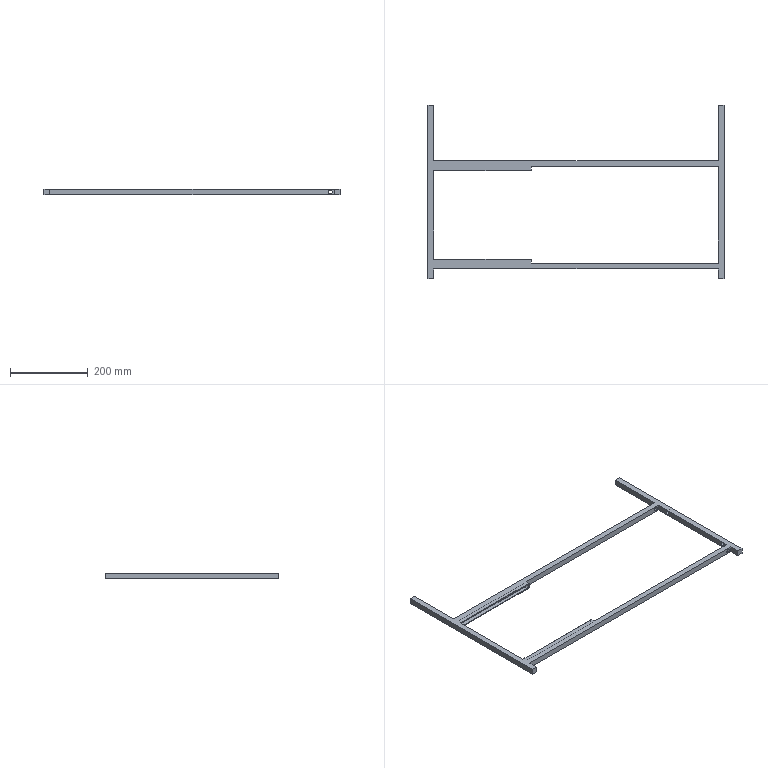Part | SolidWorks | features ICE 4, Cut 1, Extrusion 1 | 1 solid | 40 faces | box 760 x 445 x 15 mm | volume 540712 mm3 | plane 28 | cylinder 12 | commonest cylinder face diameters 10 x8 12 x4
STEP:
#1=CARTESIAN_POINT('',(727.5,-420.,-5.));
#2=VERTEX_POINT('',#1);
#3=CARTESIAN_POINT('',(727.5,-420.,5.));
#4=VERTEX_POINT('',#3);
#5=CARTESIAN_POINT('',(727.5,-420.,0.));
#6=DIRECTION('',(0.,1.,0.));
#7=DIRECTION('',(0.,0.,1.));
#8=AXIS2_PLACEMENT_3D('',#5,#6,#7);
#9=CIRCLE('',#8,5.);
#10=EDGE_CURVE('',#2,#4,#9,.T.);
#11=ORIENTED_EDGE('',*,*,#10,.F.);
#12=CARTESIAN_POINT('',(727.5,-405.,-5.));
#13=VERTEX_POINT('',#12);
#14=CARTESIAN_POINT('',(727.5,-642.5,-5.));
#15=DIRECTION('',(0.,1.,0.));
#16=VECTOR('',#15,1000.);
#17=LINE('',#14,#16);
#18=EDGE_CURVE('',#2,#13,#17,.T.);
#19=ORIENTED_EDGE('',*,*,#18,.T.);
#20=CARTESIAN_POINT('',(727.5,-405.,5.));
#21=VERTEX_POINT('',#20);
#22=CARTESIAN_POINT('',(727.5,-405.,0.));
#23=DIRECTION('',(0.,-1.,0.));
#24=DIRECTION('',(0.,0.,-1.));
#25=AXIS2_PLACEMENT_3D('',#22,#23,#24);
#26=CIRCLE('',#25,5.);
#27=EDGE_CURVE('',#21,#13,#26,.T.);
#28=ORIENTED_EDGE('',*,*,#27,.F.);
#29=CARTESIAN_POINT('',(727.5,-642.5,5.));
#30=DIRECTION('',(0.,1.,0.));
#31=VECTOR('',#30,1000.);
#32=LINE('',#29,#31);
#33=EDGE_CURVE('',#4,#21,#32,.T.);
#34=ORIENTED_EDGE('',*,*,#33,.F.);
#35=EDGE_LOOP('',(#11,#19,#28,#34));
#36=FACE_OUTER_BOUND('',#35,.T.);
#37=CARTESIAN_POINT('',(727.5,-642.5,0.));
#38=DIRECTION('',(0.,1.,0.));
#39=DIRECTION('',(0.,0.,1.));
#40=AXIS2_PLACEMENT_3D('',#37,#38,#39);
#41=CYLINDRICAL_SURFACE('',#40,5.);
#42=ADVANCED_FACE('',(#36),#41,.F.);
#43=CARTESIAN_POINT('',(727.5,-157.5,-5.));
#44=VERTEX_POINT('',#43);
#45=CARTESIAN_POINT('',(727.5,-157.5,5.));
#46=VERTEX_POINT('',#45);
#47=CARTESIAN_POINT('',(727.5,-157.5,0.));
#48=DIRECTION('',(0.,1.,0.));
#49=DIRECTION('',(0.,0.,1.));
#50=AXIS2_PLACEMENT_3D('',#47,#48,#49);
#51=CIRCLE('',#50,5.);
#52=EDGE_CURVE('',#44,#46,#51,.T.);
#53=ORIENTED_EDGE('',*,*,#52,.F.);
#54=CARTESIAN_POINT('',(727.5,-142.5,-5.));
#55=VERTEX_POINT('',#54);
#56=CARTESIAN_POINT('',(727.5,-642.5,-5.));
#57=DIRECTION('',(0.,1.,0.));
#58=VECTOR('',#57,1000.);
#59=LINE('',#56,#58);
#60=EDGE_CURVE('',#44,#55,#59,.T.);
#61=ORIENTED_EDGE('',*,*,#60,.T.);
#62=CARTESIAN_POINT('',(727.5,-142.5,5.));
#63=VERTEX_POINT('',#62);
#64=CARTESIAN_POINT('',(727.5,-142.5,0.));
#65=DIRECTION('',(0.,1.,0.));
#66=DIRECTION('',(0.,0.,1.));
#67=AXIS2_PLACEMENT_3D('',#64,#65,#66);
#68=CIRCLE('',#67,5.);
#69=EDGE_CURVE('',#55,#63,#68,.T.);
#70=ORIENTED_EDGE('',*,*,#69,.T.);
#71=CARTESIAN_POINT('',(727.5,-642.5,5.));
#72=DIRECTION('',(0.,1.,0.));
#73=VECTOR('',#72,1000.);
#74=LINE('',#71,#73);
#75=EDGE_CURVE('',#46,#63,#74,.T.);
#76=ORIENTED_EDGE('',*,*,#75,.F.);
#77=EDGE_LOOP('',(#53,#61,#70,#76));
#78=FACE_OUTER_BOUND('',#77,.T.);
#79=CARTESIAN_POINT('',(727.5,-642.5,0.));
#80=DIRECTION('',(0.,1.,0.));
#81=DIRECTION('',(0.,0.,1.));
#82=AXIS2_PLACEMENT_3D('',#79,#80,#81);
#83=CYLINDRICAL_SURFACE('',#82,5.);
#84=ADVANCED_FACE('',(#78),#83,.F.);
#85=CARTESIAN_POINT('',(752.5,-190.,-5.));
#86=VERTEX_POINT('',#85);
#87=CARTESIAN_POINT('',(752.5,-190.,5.));
#88=VERTEX_POINT('',#87);
#89=CARTESIAN_POINT('',(752.5,-190.,0.));
#90=DIRECTION('',(-1.,0.,0.));
#91=DIRECTION('',(0.,0.,-1.));
#92=AXIS2_PLACEMENT_3D('',#89,#90,#91);
#93=CIRCLE('',#92,5.);
#94=EDGE_CURVE('',#86,#88,#93,.T.);
#95=ORIENTED_EDGE('',*,*,#94,.F.);
#96=CARTESIAN_POINT('',(737.5,-190.,-5.));
#97=VERTEX_POINT('',#96);
#98=CARTESIAN_POINT('',(907.5,-190.,-5.));
#99=DIRECTION('',(-1.,0.,0.));
#100=VECTOR('',#99,1000.);
#101=LINE('',#98,#100);
#102=EDGE_CURVE('',#86,#97,#101,.T.);
#103=ORIENTED_EDGE('',*,*,#102,.T.);
#104=CARTESIAN_POINT('',(737.5,-190.,5.));
#105=VERTEX_POINT('',#104);
#106=CARTESIAN_POINT('',(737.5,-190.,0.));
#107=DIRECTION('',(1.,0.,0.));
#108=DIRECTION('',(0.,0.,1.));
#109=AXIS2_PLACEMENT_3D('',#106,#107,#108);
#110=CIRCLE('',#109,5.);
#111=EDGE_CURVE('',#105,#97,#110,.T.);
#112=ORIENTED_EDGE('',*,*,#111,.F.);
#113=CARTESIAN_POINT('',(907.5,-190.,5.));
#114=DIRECTION('',(-1.,0.,0.));
#115=VECTOR('',#114,1000.);
#116=LINE('',#113,#115);
#117=EDGE_CURVE('',#88,#105,#116,.T.);
#118=ORIENTED_EDGE('',*,*,#117,.F.);
#119=EDGE_LOOP('',(#95,#103,#112,#118));
#120=FACE_OUTER_BOUND('',#119,.T.);
#121=CARTESIAN_POINT('',(907.5,-190.,0.));
#122=DIRECTION('',(-1.,0.,0.));
#123=DIRECTION('',(0.,0.,1.));
#124=AXIS2_PLACEMENT_3D('',#121,#122,#123);
#125=CYLINDRICAL_SURFACE('',#124,5.);
#126=ADVANCED_FACE('',(#120),#125,.F.);
#127=CARTESIAN_POINT('',(752.5,-390.,-5.));
#128=VERTEX_POINT('',#127);
#129=CARTESIAN_POINT('',(752.5,-390.,5.));
#130=VERTEX_POINT('',#129);
#131=CARTESIAN_POINT('',(752.5,-390.,0.));
#132=DIRECTION('',(-1.,0.,0.));
#133=DIRECTION('',(0.,0.,-1.));
#134=AXIS2_PLACEMENT_3D('',#131,#132,#133);
#135=CIRCLE('',#134,5.);
#136=EDGE_CURVE('',#128,#130,#135,.T.);
#137=ORIENTED_EDGE('',*,*,#136,.F.);
#138=CARTESIAN_POINT('',(737.5,-390.,-5.));
#139=VERTEX_POINT('',#138);
#140=CARTESIAN_POINT('',(907.5,-390.,-5.));
#141=DIRECTION('',(-1.,0.,0.));
#142=VECTOR('',#141,1000.);
#143=LINE('',#140,#142);
#144=EDGE_CURVE('',#128,#139,#143,.T.);
#145=ORIENTED_EDGE('',*,*,#144,.T.);
#146=CARTESIAN_POINT('',(737.5,-390.,5.));
#147=VERTEX_POINT('',#146);
#148=CARTESIAN_POINT('',(737.5,-390.,0.));
#149=DIRECTION('',(1.,0.,0.));
#150=DIRECTION('',(0.,0.,1.));
#151=AXIS2_PLACEMENT_3D('',#148,#149,#150);
#152=CIRCLE('',#151,5.);
#153=EDGE_CURVE('',#147,#139,#152,.T.);
#154=ORIENTED_EDGE('',*,*,#153,.F.);
#155=CARTESIAN_POINT('',(907.5,-390.,5.));
#156=DIRECTION('',(-1.,0.,0.));
#157=VECTOR('',#156,1000.);
#158=LINE('',#155,#157);
#159=EDGE_CURVE('',#130,#147,#158,.T.);
#160=ORIENTED_EDGE('',*,*,#159,.F.);
#161=EDGE_LOOP('',(#137,#145,#154,#160));
#162=FACE_OUTER_BOUND('',#161,.T.);
#163=CARTESIAN_POINT('',(907.5,-390.,0.));
#164=DIRECTION('',(-1.,0.,0.));
#165=DIRECTION('',(0.,0.,1.));
#166=AXIS2_PLACEMENT_3D('',#163,#164,#165);
#167=CYLINDRICAL_SURFACE('',#166,5.);
#168=ADVANCED_FACE('',(#162),#167,.F.);
#169=CARTESIAN_POINT('',(727.5,-157.5,0.));
#170=DIRECTION('',(0.,1.,0.));
#171=DIRECTION('',(0.,0.,1.));
#172=AXIS2_PLACEMENT_3D('',#169,#170,#171);
#173=CIRCLE('',#172,5.);
#174=EDGE_CURVE('',#46,#44,#173,.T.);
#175=ORIENTED_EDGE('',*,*,#174,.T.);
#176=ORIENTED_EDGE('',*,*,#52,.T.);
#177=EDGE_LOOP('',(#175,#176));
#178=FACE_BOUND('',#177,.T.);
#179=CARTESIAN_POINT('',(257.5,-157.5,-7.5));
#180=VERTEX_POINT('',#179);
#181=CARTESIAN_POINT('',(257.5,-157.5,7.5));
#182=VERTEX_POINT('',#181);
#183=CARTESIAN_POINT('',(257.5,-157.5,0.));
#184=DIRECTION('',(0.,0.,1.));
#185=VECTOR('',#184,1000.);
#186=LINE('',#183,#185);
#187=EDGE_CURVE('',#180,#182,#186,.T.);
#188=ORIENTED_EDGE('',*,*,#187,.F.);
#189=CARTESIAN_POINT('',(737.5,-157.5,-7.5));
#190=VERTEX_POINT('',#189);
#191=CARTESIAN_POINT('',(758.713,-157.5,-7.5));
#192=DIRECTION('',(-1.,0.,0.));
#193=VECTOR('',#192,1000.);
#194=LINE('',#191,#193);
#195=EDGE_CURVE('',#190,#180,#194,.T.);
#196=ORIENTED_EDGE('',*,*,#195,.F.);
#197=CARTESIAN_POINT('',(737.5,-157.5,7.5));
#198=VERTEX_POINT('',#197);
#199=CARTESIAN_POINT('',(737.5,-157.5,7.5));
#200=DIRECTION('',(0.,0.,1.));
#201=VECTOR('',#200,1000.);
#202=LINE('',#199,#201);
#203=EDGE_CURVE('',#190,#198,#202,.T.);
#204=ORIENTED_EDGE('',*,*,#203,.T.);
#205=CARTESIAN_POINT('',(758.713,-157.5,7.5));
#206=DIRECTION('',(-1.,0.,0.));
#207=VECTOR('',#206,1000.);
#208=LINE('',#205,#207);
#209=EDGE_CURVE('',#198,#182,#208,.T.);
#210=ORIENTED_EDGE('',*,*,#209,.T.);
#211=EDGE_LOOP('',(#188,#196,#204,#210));
#212=FACE_OUTER_BOUND('',#211,.T.);
#213=CARTESIAN_POINT('',(758.713,-157.5,7.5));
#214=DIRECTION('',(0.,1.,0.));
#215=DIRECTION('',(0.,0.,1.));
#216=AXIS2_PLACEMENT_3D('',#213,#214,#215);
#217=PLANE('',#216);
#218=ADVANCED_FACE('',(#178,#212),#217,.F.);
#219=ORIENTED_EDGE('',*,*,#27,.T.);
#220=CARTESIAN_POINT('',(727.5,-405.,0.));
#221=DIRECTION('',(0.,-1.,0.));
#222=DIRECTION('',(0.,0.,-1.));
#223=AXIS2_PLACEMENT_3D('',#220,#221,#222);
#224=CIRCLE('',#223,5.);
#225=EDGE_CURVE('',#13,#21,#224,.T.);
#226=ORIENTED_EDGE('',*,*,#225,.T.);
#227=EDGE_LOOP('',(#219,#226));
#228=FACE_BOUND('',#227,.T.);
#229=CARTESIAN_POINT('',(737.5,-405.,-7.5));
#230=VERTEX_POINT('',#229);
#231=CARTESIAN_POINT('',(257.5,-405.,-7.5));
#232=VERTEX_POINT('',#231);
#233=CARTESIAN_POINT('',(758.713,-405.,-7.5));
#234=DIRECTION('',(-1.,0.,0.));
#235=VECTOR('',#234,1000.);
#236=LINE('',#233,#235);
#237=EDGE_CURVE('',#230,#232,#236,.T.);
#238=ORIENTED_EDGE('',*,*,#237,.T.);
#239=CARTESIAN_POINT('',(257.5,-405.,7.5));
#240=VERTEX_POINT('',#239);
#241=CARTESIAN_POINT('',(257.5,-405.,0.));
#242=DIRECTION('',(0.,0.,1.));
#243=VECTOR('',#242,1000.);
#244=LINE('',#241,#243);
#245=EDGE_CURVE('',#232,#240,#244,.T.);
#246=ORIENTED_EDGE('',*,*,#245,.T.);
#247=CARTESIAN_POINT('',(737.5,-405.,7.5));
#248=VERTEX_POINT('',#247);
#249=CARTESIAN_POINT('',(758.713,-405.,7.5));
#250=DIRECTION('',(-1.,0.,0.));
#251=VECTOR('',#250,1000.);
#252=LINE('',#249,#251);
#253=EDGE_CURVE('',#248,#240,#252,.T.);
#254=ORIENTED_EDGE('',*,*,#253,.F.);
#255=CARTESIAN_POINT('',(737.5,-405.,7.5));
#256=DIRECTION('',(0.,0.,-1.));
#257=VECTOR('',#256,1000.);
#258=LINE('',#255,#257);
#259=EDGE_CURVE('',#248,#230,#258,.T.);
#260=ORIENTED_EDGE('',*,*,#259,.T.);
#261=EDGE_LOOP('',(#238,#246,#254,#260));
#262=FACE_OUTER_BOUND('',#261,.T.);
#263=CARTESIAN_POINT('',(758.713,-405.,7.5));
#264=DIRECTION('',(0.,-1.,0.));
#265=DIRECTION('',(0.,0.,-1.));
#266=AXIS2_PLACEMENT_3D('',#263,#264,#265);
#267=PLANE('',#266);
#268=ADVANCED_FACE('',(#228,#262),#267,.F.);
#269=CARTESIAN_POINT('',(7.5,-167.5,7.5));
#270=VERTEX_POINT('',#269);
#271=CARTESIAN_POINT('',(7.5,-167.5,-7.5));
#272=VERTEX_POINT('',#271);
#273=CARTESIAN_POINT('',(7.5,-167.5,0.));
#274=DIRECTION('',(0.,0.,-1.));
#275=VECTOR('',#274,1000.);
#276=LINE('',#273,#275);
#277=EDGE_CURVE('',#270,#272,#276,.T.);
#278=ORIENTED_EDGE('',*,*,#277,.F.);
#279=CARTESIAN_POINT('',(7.5,-395.,7.5));
#280=VERTEX_POINT('',#279);
#281=CARTESIAN_POINT('',(7.5,-445.,7.5));
#282=DIRECTION('',(0.,1.,0.));
#283=VECTOR('',#282,1000.);
#284=LINE('',#281,#283);
#285=EDGE_CURVE('',#280,#270,#284,.T.);
#286=ORIENTED_EDGE('',*,*,#285,.F.);
#287=CARTESIAN_POINT('',(7.5,-395.,-7.5));
#288=VERTEX_POINT('',#287);
#289=CARTESIAN_POINT('',(7.5,-395.,0.));
#290=DIRECTION('',(0.,0.,1.));
#291=VECTOR('',#290,1000.);
#292=LINE('',#289,#291);
#293=EDGE_CURVE('',#288,#280,#292,.T.);
#294=ORIENTED_EDGE('',*,*,#293,.F.);
#295=CARTESIAN_POINT('',(7.5,-445.,-7.5));
#296=DIRECTION('',(0.,1.,0.));
#297=VECTOR('',#296,1000.);
#298=LINE('',#295,#297);
#299=EDGE_CURVE('',#288,#272,#298,.T.);
#300=ORIENTED_EDGE('',*,*,#299,.T.);
#301=EDGE_LOOP('',(#278,#286,#294,#300));
#302=FACE_OUTER_BOUND('',#301,.T.);
#303=CARTESIAN_POINT('',(7.5,-445.,-7.5));
#304=DIRECTION('',(1.,0.,0.));
#305=DIRECTION('',(0.,0.,-1.));
#306=AXIS2_PLACEMENT_3D('',#303,#304,#305);
#307=PLANE('',#306);
#308=ADVANCED_FACE('',(#302),#307,.T.);
#309=CARTESIAN_POINT('',(7.5,-142.5,7.5));
#310=VERTEX_POINT('',#309);
#311=CARTESIAN_POINT('',(7.5,0.,7.5));
#312=VERTEX_POINT('',#311);
#313=CARTESIAN_POINT('',(7.5,-445.,7.5));
#314=DIRECTION('',(0.,1.,0.));
#315=VECTOR('',#314,1000.);
#316=LINE('',#313,#315);
#317=EDGE_CURVE('',#310,#312,#316,.T.);
#318=ORIENTED_EDGE('',*,*,#317,.F.);
#319=CARTESIAN_POINT('',(7.5,-142.5,-7.5));
#320=VERTEX_POINT('',#319);
#321=CARTESIAN_POINT('',(7.5,-142.5,7.5));
#322=DIRECTION('',(0.,0.,1.));
#323=VECTOR('',#322,1000.);
#324=LINE('',#321,#323);
#325=EDGE_CURVE('',#320,#310,#324,.T.);
#326=ORIENTED_EDGE('',*,*,#325,.F.);
#327=CARTESIAN_POINT('',(7.5,0.,-7.5));
#328=VERTEX_POINT('',#327);
#329=CARTESIAN_POINT('',(7.5,-445.,-7.5));
#330=DIRECTION('',(0.,1.,0.));
#331=VECTOR('',#330,1000.);
#332=LINE('',#329,#331);
#333=EDGE_CURVE('',#320,#328,#332,.T.);
#334=ORIENTED_EDGE('',*,*,#333,.T.);
#335=CARTESIAN_POINT('',(7.5,0.,-7.5));
#336=DIRECTION('',(0.,0.,-1.));
#337=VECTOR('',#336,1000.);
#338=LINE('',#335,#337);
#339=EDGE_CURVE('',#312,#328,#338,.T.);
#340=ORIENTED_EDGE('',*,*,#339,.F.);
#341=EDGE_LOOP('',(#318,#326,#334,#340));
#342=FACE_OUTER_BOUND('',#341,.T.);
#343=CARTESIAN_POINT('',(7.5,-445.,-7.5));
#344=DIRECTION('',(1.,0.,0.));
#345=DIRECTION('',(0.,0.,-1.));
#346=AXIS2_PLACEMENT_3D('',#343,#344,#345);
#347=PLANE('',#346);
#348=ADVANCED_FACE('',(#342),#347,.T.);
#349=ORIENTED_EDGE('',*,*,#111,.T.);
#350=CARTESIAN_POINT('',(737.5,-190.,0.));
#351=DIRECTION('',(1.,0.,0.));
#352=DIRECTION('',(0.,0.,1.));
#353=AXIS2_PLACEMENT_3D('',#350,#351,#352);
#354=CIRCLE('',#353,5.);
#355=EDGE_CURVE('',#97,#105,#354,.T.);
#356=ORIENTED_EDGE('',*,*,#355,.T.);
#357=EDGE_LOOP('',(#349,#356));
#358=FACE_BOUND('',#357,.T.);
#359=ORIENTED_EDGE('',*,*,#153,.T.);
#360=CARTESIAN_POINT('',(737.5,-390.,0.));
#361=DIRECTION('',(1.,0.,0.));
#362=DIRECTION('',(0.,0.,1.));
#363=AXIS2_PLACEMENT_3D('',#360,#361,#362);
#364=CIRCLE('',#363,5.);
#365=EDGE_CURVE('',#139,#147,#364,.T.);
#366=ORIENTED_EDGE('',*,*,#365,.T.);
#367=EDGE_LOOP('',(#359,#366));
#368=FACE_BOUND('',#367,.T.);
#369=CARTESIAN_POINT('',(737.5,-445.,7.5));
#370=DIRECTION('',(0.,1.,0.));
#371=VECTOR('',#370,1000.);
#372=LINE('',#369,#371);
#373=EDGE_CURVE('',#248,#198,#372,.T.);
#374=ORIENTED_EDGE('',*,*,#373,.T.);
#375=ORIENTED_EDGE('',*,*,#203,.F.);
#376=CARTESIAN_POINT('',(737.5,-445.,-7.5));
#377=DIRECTION('',(0.,1.,0.));
#378=VECTOR('',#377,1000.);
#379=LINE('',#376,#378);
#380=EDGE_CURVE('',#230,#190,#379,.T.);
#381=ORIENTED_EDGE('',*,*,#380,.F.);
#382=ORIENTED_EDGE('',*,*,#259,.F.);
#383=EDGE_LOOP('',(#374,#375,#381,#382));
#384=FACE_OUTER_BOUND('',#383,.T.);
#385=CARTESIAN_POINT('',(737.5,-445.,-7.5));
#386=DIRECTION('',(-1.,0.,0.));
#387=DIRECTION('',(0.,0.,1.));
#388=AXIS2_PLACEMENT_3D('',#385,#386,#387);
#389=PLANE('',#388);
#390=ADVANCED_FACE('',(#358,#368,#384),#389,.T.);
#391=CARTESIAN_POINT('',(737.5,-142.5,-7.5));
#392=VERTEX_POINT('',#391);
#393=CARTESIAN_POINT('',(737.5,0.,-7.5));
#394=VERTEX_POINT('',#393);
#395=CARTESIAN_POINT('',(737.5,-445.,-7.5));
#396=DIRECTION('',(0.,1.,0.));
#397=VECTOR('',#396,1000.);
#398=LINE('',#395,#397);
#399=EDGE_CURVE('',#392,#394,#398,.T.);
#400=ORIENTED_EDGE('',*,*,#399,.F.);
#401=CARTESIAN_POINT('',(737.5,-142.5,7.5));
#402=VERTEX_POINT('',#401);
#403=CARTESIAN_POINT('',(737.5,-142.5,7.5));
#404=DIRECTION('',(0.,0.,-1.));
#405=VECTOR('',#404,1000.);
#406=LINE('',#403,#405);
#407=EDGE_CURVE('',#402,#392,#406,.T.);
#408=ORIENTED_EDGE('',*,*,#407,.F.);
#409=CARTESIAN_POINT('',(737.5,0.,7.5));
#410=VERTEX_POINT('',#409);
#411=CARTESIAN_POINT('',(737.5,-445.,7.5));
#412=DIRECTION('',(0.,1.,0.));
#413=VECTOR('',#412,1000.);
#414=LINE('',#411,#413);
#415=EDGE_CURVE('',#402,#410,#414,.T.);
#416=ORIENTED_EDGE('',*,*,#415,.T.);
#417=CARTESIAN_POINT('',(737.5,0.,-7.5));
#418=DIRECTION('',(0.,0.,1.));
#419=VECTOR('',#418,1000.);
#420=LINE('',#417,#419);
#421=EDGE_CURVE('',#394,#410,#420,.T.);
#422=ORIENTED_EDGE('',*,*,#421,.F.);
#423=EDGE_LOOP('',(#400,#408,#416,#422));
#424=FACE_OUTER_BOUND('',#423,.T.);
#425=CARTESIAN_POINT('',(737.5,-445.,-7.5));
#426=DIRECTION('',(-1.,0.,0.));
#427=DIRECTION('',(0.,0.,1.));
#428=AXIS2_PLACEMENT_3D('',#425,#426,#427);
#429=PLANE('',#428);
#430=ADVANCED_FACE('',(#424),#429,.T.);
#431=CARTESIAN_POINT('',(7.5,-420.,7.5));
#432=VERTEX_POINT('',#431);
#433=CARTESIAN_POINT('',(7.5,-420.,-7.5));
#434=VERTEX_POINT('',#433);
#435=CARTESIAN_POINT('',(7.5,-420.,7.5));
#436=DIRECTION('',(0.,0.,-1.));
#437=VECTOR('',#436,1000.);
#438=LINE('',#435,#437);
#439=EDGE_CURVE('',#432,#434,#438,.T.);
#440=ORIENTED_EDGE('',*,*,#439,.F.);
#441=CARTESIAN_POINT('',(7.5,-445.,7.5));
#442=VERTEX_POINT('',#441);
#443=CARTESIAN_POINT('',(7.5,-445.,7.5));
#444=DIRECTION('',(0.,1.,0.));
#445=VECTOR('',#444,1000.);
#446=LINE('',#443,#445);
#447=EDGE_CURVE('',#442,#432,#446,.T.);
#448=ORIENTED_EDGE('',*,*,#447,.F.);
#449=CARTESIAN_POINT('',(7.5,-445.,-7.5));
#450=VERTEX_POINT('',#449);
#451=CARTESIAN_POINT('',(7.5,-445.,-7.5));
#452=DIRECTION('',(0.,0.,-1.));
#453=VECTOR('',#452,1000.);
#454=LINE('',#451,#453);
#455=EDGE_CURVE('',#442,#450,#454,.T.);
#456=ORIENTED_EDGE('',*,*,#455,.T.);
#457=CARTESIAN_POINT('',(7.5,-445.,-7.5));
#458=DIRECTION('',(0.,1.,0.));
#459=VECTOR('',#458,1000.);
#460=LINE('',#457,#459);
#461=EDGE_CURVE('',#450,#434,#460,.T.);
#462=ORIENTED_EDGE('',*,*,#461,.T.);
#463=EDGE_LOOP('',(#440,#448,#456,#462));
#464=FACE_OUTER_BOUND('',#463,.T.);
#465=CARTESIAN_POINT('',(7.5,-445.,-7.5));
#466=DIRECTION('',(1.,0.,0.));
#467=DIRECTION('',(0.,0.,-1.));
#468=AXIS2_PLACEMENT_3D('',#465,#466,#467);
#469=PLANE('',#468);
#470=ADVANCED_FACE('',(#464),#469,.T.);
#471=CARTESIAN_POINT('',(257.5,-395.,7.5));
#472=VERTEX_POINT('',#471);
#473=CARTESIAN_POINT('',(0.,-395.,7.5));
#474=DIRECTION('',(1.,0.,0.));
#475=VECTOR('',#474,1000.);
#476=LINE('',#473,#475);
#477=EDGE_CURVE('',#280,#472,#476,.T.);
#478=ORIENTED_EDGE('',*,*,#477,.F.);
#479=ORIENTED_EDGE('',*,*,#285,.T.);
#480=CARTESIAN_POINT('',(257.5,-167.5,7.5));
#481=VERTEX_POINT('',#480);
#482=CARTESIAN_POINT('',(0.,-167.5,7.5));
#483=DIRECTION('',(-1.,0.,0.));
#484=VECTOR('',#483,1000.);
#485=LINE('',#482,#484);
#486=EDGE_CURVE('',#481,#270,#485,.T.);
#487=ORIENTED_EDGE('',*,*,#486,.F.);
#488=CARTESIAN_POINT('',(257.5,-167.5,7.5));
#489=DIRECTION('',(0.,1.,0.));
#490=VECTOR('',#489,1000.);
#491=LINE('',#488,#490);
#492=EDGE_CURVE('',#481,#182,#491,.T.);
#493=ORIENTED_EDGE('',*,*,#492,.T.);
#494=ORIENTED_EDGE('',*,*,#209,.F.);
#495=ORIENTED_EDGE('',*,*,#373,.F.);
#496=ORIENTED_EDGE('',*,*,#253,.T.);
#497=CARTESIAN_POINT('',(257.5,-395.,7.5));
#498=DIRECTION('',(0.,-1.,0.));
#499=VECTOR('',#498,1000.);
#500=LINE('',#497,#499);
#501=EDGE_CURVE('',#472,#240,#500,.T.);
#502=ORIENTED_EDGE('',*,*,#501,.F.);
#503=EDGE_LOOP('',(#478,#479,#487,#493,#494,#495,#496,#502));
#504=FACE_BOUND('',#503,.T.);
#505=CARTESIAN_POINT('',(-7.5,0.,7.5));
#506=VERTEX_POINT('',#505);
#507=CARTESIAN_POINT('',(-7.5,0.,7.5));
#508=DIRECTION('',(1.,0.,0.));
#509=VECTOR('',#508,1000.);
#510=LINE('',#507,#509);
#511=EDGE_CURVE('',#506,#312,#510,.T.);
#512=ORIENTED_EDGE('',*,*,#511,.F.);
#513=CARTESIAN_POINT('',(-7.5,-445.,7.5));
#514=VERTEX_POINT('',#513);
#515=CARTESIAN_POINT('',(-7.5,-445.,7.5));
#516=DIRECTION('',(0.,1.,0.));
#517=VECTOR('',#516,1000.);
#518=LINE('',#515,#517);
#519=EDGE_CURVE('',#514,#506,#518,.T.);
#520=ORIENTED_EDGE('',*,*,#519,.F.);
#521=CARTESIAN_POINT('',(-7.5,-445.,7.5));
#522=DIRECTION('',(1.,0.,0.));
#523=VECTOR('',#522,1000.);
#524=LINE('',#521,#523);
#525=EDGE_CURVE('',#514,#442,#524,.T.);
#526=ORIENTED_EDGE('',*,*,#525,.T.);
#527=ORIENTED_EDGE('',*,*,#447,.T.);
#528=CARTESIAN_POINT('',(737.5,-420.,7.5));
#529=VERTEX_POINT('',#528);
#530=CARTESIAN_POINT('',(758.713,-420.,7.5));
#531=DIRECTION('',(-1.,0.,0.));
#532=VECTOR('',#531,1000.);
#533=LINE('',#530,#532);
#534=EDGE_CURVE('',#529,#432,#533,.T.);
#535=ORIENTED_EDGE('',*,*,#534,.F.);
#536=CARTESIAN_POINT('',(737.5,-445.,7.5));
#537=VERTEX_POINT('',#536);
#538=CARTESIAN_POINT('',(737.5,-445.,7.5));
#539=DIRECTION('',(0.,1.,0.));
#540=VECTOR('',#539,1000.);
#541=LINE('',#538,#540);
#542=EDGE_CURVE('',#537,#529,#541,.T.);
#543=ORIENTED_EDGE('',*,*,#542,.F.);
#544=CARTESIAN_POINT('',(752.5,-445.,7.5));
#545=VERTEX_POINT('',#544);
#546=CARTESIAN_POINT('',(752.5,-445.,7.5));
#547=DIRECTION('',(1.,0.,0.));
#548=VECTOR('',#547,1000.);
#549=LINE('',#546,#548);
#550=EDGE_CURVE('',#537,#545,#549,.T.);
#551=ORIENTED_EDGE('',*,*,#550,.T.);
#552=CARTESIAN_POINT('',(752.5,0.,7.5));
#553=VERTEX_POINT('',#552);
#554=CARTESIAN_POINT('',(752.5,-445.,7.5));
#555=DIRECTION('',(0.,1.,0.));
#556=VECTOR('',#555,1000.);
#557=LINE('',#554,#556);
#558=EDGE_CURVE('',#545,#553,#557,.T.);
#559=ORIENTED_EDGE('',*,*,#558,.T.);
#560=CARTESIAN_POINT('',(752.5,0.,7.5));
#561=DIRECTION('',(1.,0.,0.));
#562=VECTOR('',#561,1000.);
#563=LINE('',#560,#562);
#564=EDGE_CURVE('',#410,#553,#563,.T.);
#565=ORIENTED_EDGE('',*,*,#564,.F.);
#566=ORIENTED_EDGE('',*,*,#415,.F.);
#567=CARTESIAN_POINT('',(758.713,-142.5,7.5));
#568=DIRECTION('',(-1.,0.,0.));
#569=VECTOR('',#568,1000.);
#570=LINE('',#567,#569);
#571=EDGE_CURVE('',#402,#310,#570,.T.);
#572=ORIENTED_EDGE('',*,*,#571,.T.);
#573=ORIENTED_EDGE('',*,*,#317,.T.);
#574=EDGE_LOOP('',(#512,#520,#526,#527,#535,#543,#551,#559,#565,#566,#572,#573));
#575=FACE_OUTER_BOUND('',#574,.T.);
#576=CARTESIAN_POINT('',(-7.5,-445.,7.5));
#577=DIRECTION('',(0.,0.,1.));
#578=DIRECTION('',(1.,0.,0.));
#579=AXIS2_PLACEMENT_3D('',#576,#577,#578);
#580=PLANE('',#579);
#581=ADVANCED_FACE('',(#504,#575),#580,.T.);
#582=CARTESIAN_POINT('',(-7.5,0.,-7.5));
#583=VERTEX_POINT('',#582);
#584=CARTESIAN_POINT('',(-7.5,0.,-7.5));
#585=DIRECTION('',(0.,0.,1.));
#586=VECTOR('',#585,1000.);
#587=LINE('',#584,#586);
#588=EDGE_CURVE('',#583,#506,#587,.T.);
#589=ORIENTED_EDGE('',*,*,#588,.F.);
#590=CARTESIAN_POINT('',(-7.5,-445.,-7.5));
#591=VERTEX_POINT('',#590);
#592=CARTESIAN_POINT('',(-7.5,-445.,-7.5));
#593=DIRECTION('',(0.,1.,0.));
#594=VECTOR('',#593,1000.);
#595=LINE('',#592,#594);
#596=EDGE_CURVE('',#591,#583,#595,.T.);
#597=ORIENTED_EDGE('',*,*,#596,.F.);
#598=CARTESIAN_POINT('',(-7.5,-445.,-7.5));
#599=DIRECTION('',(0.,0.,1.));
#600=VECTOR('',#599,1000.);
#601=LINE('',#598,#600);
#602=EDGE_CURVE('',#591,#514,#601,.T.);
#603=ORIENTED_EDGE('',*,*,#602,.T.);
#604=ORIENTED_EDGE('',*,*,#519,.T.);
#605=EDGE_LOOP('',(#589,#597,#603,#604));
#606=FACE_OUTER_BOUND('',#605,.T.);
#607=CARTESIAN_POINT('',(-7.5,-445.,-7.5));
#608=DIRECTION('',(-1.,0.,0.));
#609=DIRECTION('',(0.,0.,1.));
#610=AXIS2_PLACEMENT_3D('',#607,#608,#609);
#611=PLANE('',#610);
#612=ADVANCED_FACE('',(#606),#611,.T.);
#613=ORIENTED_EDGE('',*,*,#299,.F.);
#614=CARTESIAN_POINT('',(257.5,-395.,-7.5));
#615=VERTEX_POINT('',#614);
#616=CARTESIAN_POINT('',(0.,-395.,-7.5));
#617=DIRECTION('',(-1.,0.,0.));
#618=VECTOR('',#617,1000.);
#619=LINE('',#616,#618);
#620=EDGE_CURVE('',#615,#288,#619,.T.);
#621=ORIENTED_EDGE('',*,*,#620,.F.);
#622=CARTESIAN_POINT('',(257.5,-395.,-7.5));
#623=DIRECTION('',(0.,-1.,0.));
#624=VECTOR('',#623,1000.);
#625=LINE('',#622,#624);
#626=EDGE_CURVE('',#615,#232,#625,.T.);
#627=ORIENTED_EDGE('',*,*,#626,.T.);
#628=ORIENTED_EDGE('',*,*,#237,.F.);
#629=ORIENTED_EDGE('',*,*,#380,.T.);
#630=ORIENTED_EDGE('',*,*,#195,.T.);
#631=CARTESIAN_POINT('',(257.5,-167.5,-7.5));
#632=VERTEX_POINT('',#631);
#633=CARTESIAN_POINT('',(257.5,-167.5,-7.5));
#634=DIRECTION('',(0.,1.,0.));
#635=VECTOR('',#634,1000.);
#636=LINE('',#633,#635);
#637=EDGE_CURVE('',#632,#180,#636,.T.);
#638=ORIENTED_EDGE('',*,*,#637,.F.);
#639=CARTESIAN_POINT('',(0.,-167.5,-7.5));
#640=DIRECTION('',(1.,0.,0.));
#641=VECTOR('',#640,1000.);
#642=LINE('',#639,#641);
#643=EDGE_CURVE('',#272,#632,#642,.T.);
#644=ORIENTED_EDGE('',*,*,#643,.F.);
#645=EDGE_LOOP('',(#613,#621,#627,#628,#629,#630,#638,#644));
#646=FACE_BOUND('',#645,.T.);
#647=ORIENTED_EDGE('',*,*,#333,.F.);
#648=CARTESIAN_POINT('',(758.713,-142.5,-7.5));
#649=DIRECTION('',(-1.,0.,0.));
#650=VECTOR('',#649,1000.);
#651=LINE('',#648,#650);
#652=EDGE_CURVE('',#392,#320,#651,.T.);
#653=ORIENTED_EDGE('',*,*,#652,.F.);
#654=ORIENTED_EDGE('',*,*,#399,.T.);
#655=CARTESIAN_POINT('',(752.5,0.,-7.5));
#656=VERTEX_POINT('',#655);
#657=CARTESIAN_POINT('',(752.5,0.,-7.5));
#658=DIRECTION('',(-1.,0.,0.));
#659=VECTOR('',#658,1000.);
#660=LINE('',#657,#659);
#661=EDGE_CURVE('',#656,#394,#660,.T.);
#662=ORIENTED_EDGE('',*,*,#661,.F.);
#663=CARTESIAN_POINT('',(752.5,-445.,-7.5));
#664=VERTEX_POINT('',#663);
#665=CARTESIAN_POINT('',(752.5,-445.,-7.5));
#666=DIRECTION('',(0.,1.,0.));
#667=VECTOR('',#666,1000.);
#668=LINE('',#665,#667);
#669=EDGE_CURVE('',#664,#656,#668,.T.);
#670=ORIENTED_EDGE('',*,*,#669,.F.);
#671=CARTESIAN_POINT('',(737.5,-445.,-7.5));
#672=VERTEX_POINT('',#671);
#673=CARTESIAN_POINT('',(752.5,-445.,-7.5));
#674=DIRECTION('',(-1.,0.,0.));
#675=VECTOR('',#674,1000.);
#676=LINE('',#673,#675);
#677=EDGE_CURVE('',#664,#672,#676,.T.);
#678=ORIENTED_EDGE('',*,*,#677,.T.);
#679=CARTESIAN_POINT('',(737.5,-420.,-7.5));
#680=VERTEX_POINT('',#679);
#681=CARTESIAN_POINT('',(737.5,-445.,-7.5));
#682=DIRECTION('',(0.,1.,0.));
#683=VECTOR('',#682,1000.);
#684=LINE('',#681,#683);
#685=EDGE_CURVE('',#672,#680,#684,.T.);
#686=ORIENTED_EDGE('',*,*,#685,.T.);
#687=CARTESIAN_POINT('',(758.713,-420.,-7.5));
#688=DIRECTION('',(-1.,0.,0.));
#689=VECTOR('',#688,1000.);
#690=LINE('',#687,#689);
#691=EDGE_CURVE('',#680,#434,#690,.T.);
#692=ORIENTED_EDGE('',*,*,#691,.T.);
#693=ORIENTED_EDGE('',*,*,#461,.F.);
#694=CARTESIAN_POINT('',(-7.5,-445.,-7.5));
#695=DIRECTION('',(-1.,0.,0.));
#696=VECTOR('',#695,1000.);
#697=LINE('',#694,#696);
#698=EDGE_CURVE('',#450,#591,#697,.T.);
#699=ORIENTED_EDGE('',*,*,#698,.T.);
#700=ORIENTED_EDGE('',*,*,#596,.T.);
#701=CARTESIAN_POINT('',(-7.5,0.,-7.5));
#702=DIRECTION('',(-1.,0.,0.));
#703=VECTOR('',#702,1000.);
#704=LINE('',#701,#703);
#705=EDGE_CURVE('',#328,#583,#704,.T.);
#706=ORIENTED_EDGE('',*,*,#705,.F.);
#707=EDGE_LOOP('',(#647,#653,#654,#662,#670,#678,#686,#692,#693,#699,#700,#706));
#708=FACE_OUTER_BOUND('',#707,.T.);
#709=CARTESIAN_POINT('',(-7.5,-445.,-7.5));
#710=DIRECTION('',(0.,0.,-1.));
#711=DIRECTION('',(-1.,0.,0.));
#712=AXIS2_PLACEMENT_3D('',#709,#710,#711);
#713=PLANE('',#712);
#714=ADVANCED_FACE('',(#646,#708),#713,.T.);
#715=ORIENTED_EDGE('',*,*,#455,.F.);
#716=ORIENTED_EDGE('',*,*,#525,.F.);
#717=ORIENTED_EDGE('',*,*,#602,.F.);
#718=ORIENTED_EDGE('',*,*,#698,.F.);
#719=EDGE_LOOP('',(#715,#716,#717,#718));
#720=FACE_OUTER_BOUND('',#719,.T.);
#721=CARTESIAN_POINT('',(0.,-445.,0.));
#722=DIRECTION('',(0.,1.,0.));
#723=DIRECTION('',(0.,0.,1.));
#724=AXIS2_PLACEMENT_3D('',#721,#722,#723);
#725=PLANE('',#724);
#726=ADVANCED_FACE('',(#720),#725,.F.);
#727=ORIENTED_EDGE('',*,*,#339,.T.);
#728=ORIENTED_EDGE('',*,*,#705,.T.);
#729=ORIENTED_EDGE('',*,*,#588,.T.);
#730=ORIENTED_EDGE('',*,*,#511,.T.);
#731=EDGE_LOOP('',(#727,#728,#729,#730));
#732=FACE_OUTER_BOUND('',#731,.T.);
#733=CARTESIAN_POINT('',(0.,0.,0.));
#734=DIRECTION('',(0.,1.,0.));
#735=DIRECTION('',(0.,0.,1.));
#736=AXIS2_PLACEMENT_3D('',#733,#734,#735);
#737=PLANE('',#736);
#738=ADVANCED_FACE('',(#732),#737,.T.);
#739=CARTESIAN_POINT('',(727.5,-420.,0.));
#740=DIRECTION('',(0.,1.,0.));
#741=DIRECTION('',(0.,0.,1.));
#742=AXIS2_PLACEMENT_3D('',#739,#740,#741);
#743=CIRCLE('',#742,5.);
#744=EDGE_CURVE('',#4,#2,#743,.T.);
#745=ORIENTED_EDGE('',*,*,#744,.T.);
#746=ORIENTED_EDGE('',*,*,#10,.T.);
#747=EDGE_LOOP('',(#745,#746));
#748=FACE_BOUND('',#747,.T.);
#749=ORIENTED_EDGE('',*,*,#691,.F.);
#750=CARTESIAN_POINT('',(737.5,-420.,7.5));
#751=DIRECTION('',(0.,0.,1.));
#752=VECTOR('',#751,1000.);
#753=LINE('',#750,#752);
#754=EDGE_CURVE('',#680,#529,#753,.T.);
#755=ORIENTED_EDGE('',*,*,#754,.T.);
#756=ORIENTED_EDGE('',*,*,#534,.T.);
#757=ORIENTED_EDGE('',*,*,#439,.T.);
#758=EDGE_LOOP('',(#749,#755,#756,#757));
#759=FACE_OUTER_BOUND('',#758,.T.);
#760=CARTESIAN_POINT('',(758.713,-420.,7.5));
#761=DIRECTION('',(0.,1.,0.));
#762=DIRECTION('',(0.,0.,1.));
#763=AXIS2_PLACEMENT_3D('',#760,#761,#762);
#764=PLANE('',#763);
#765=ADVANCED_FACE('',(#748,#759),#764,.F.);
#766=ORIENTED_EDGE('',*,*,#754,.F.);
#767=ORIENTED_EDGE('',*,*,#685,.F.);
#768=CARTESIAN_POINT('',(737.5,-445.,-7.5));
#769=DIRECTION('',(0.,0.,1.));
#770=VECTOR('',#769,1000.);
#771=LINE('',#768,#770);
#772=EDGE_CURVE('',#672,#537,#771,.T.);
#773=ORIENTED_EDGE('',*,*,#772,.T.);
#774=ORIENTED_EDGE('',*,*,#542,.T.);
#775=EDGE_LOOP('',(#766,#767,#773,#774));
#776=FACE_OUTER_BOUND('',#775,.T.);
#777=CARTESIAN_POINT('',(737.5,-445.,-7.5));
#778=DIRECTION('',(-1.,0.,0.));
#779=DIRECTION('',(0.,0.,1.));
#780=AXIS2_PLACEMENT_3D('',#777,#778,#779);
#781=PLANE('',#780);
#782=ADVANCED_FACE('',(#776),#781,.T.);
#783=CARTESIAN_POINT('',(752.5,-190.,0.));
#784=DIRECTION('',(-1.,0.,0.));
#785=DIRECTION('',(0.,0.,-1.));
#786=AXIS2_PLACEMENT_3D('',#783,#784,#785);
#787=CIRCLE('',#786,5.);
#788=EDGE_CURVE('',#88,#86,#787,.T.);
#789=ORIENTED_EDGE('',*,*,#788,.T.);
#790=ORIENTED_EDGE('',*,*,#94,.T.);
#791=EDGE_LOOP('',(#789,#790));
#792=FACE_BOUND('',#791,.T.);
#793=CARTESIAN_POINT('',(752.5,-390.,0.));
#794=DIRECTION('',(-1.,0.,0.));
#795=DIRECTION('',(0.,0.,-1.));
#796=AXIS2_PLACEMENT_3D('',#793,#794,#795);
#797=CIRCLE('',#796,5.);
#798=EDGE_CURVE('',#130,#128,#797,.T.);
#799=ORIENTED_EDGE('',*,*,#798,.T.);
#800=ORIENTED_EDGE('',*,*,#136,.T.);
#801=EDGE_LOOP('',(#799,#800));
#802=FACE_BOUND('',#801,.T.);
#803=CARTESIAN_POINT('',(752.5,0.,-7.5));
#804=DIRECTION('',(0.,0.,-1.));
#805=VECTOR('',#804,1000.);
#806=LINE('',#803,#805);
#807=EDGE_CURVE('',#553,#656,#806,.T.);
#808=ORIENTED_EDGE('',*,*,#807,.F.);
#809=ORIENTED_EDGE('',*,*,#558,.F.);
#810=CARTESIAN_POINT('',(752.5,-445.,-7.5));
#811=DIRECTION('',(0.,0.,-1.));
#812=VECTOR('',#811,1000.);
#813=LINE('',#810,#812);
#814=EDGE_CURVE('',#545,#664,#813,.T.);
#815=ORIENTED_EDGE('',*,*,#814,.T.);
#816=ORIENTED_EDGE('',*,*,#669,.T.);
#817=EDGE_LOOP('',(#808,#809,#815,#816));
#818=FACE_OUTER_BOUND('',#817,.T.);
#819=CARTESIAN_POINT('',(752.5,-445.,-7.5));
#820=DIRECTION('',(1.,0.,0.));
#821=DIRECTION('',(0.,0.,-1.));
#822=AXIS2_PLACEMENT_3D('',#819,#820,#821);
#823=PLANE('',#822);
#824=ADVANCED_FACE('',(#792,#802,#818),#823,.T.);
#825=ORIENTED_EDGE('',*,*,#814,.F.);
#826=ORIENTED_EDGE('',*,*,#550,.F.);
#827=ORIENTED_EDGE('',*,*,#772,.F.);
#828=ORIENTED_EDGE('',*,*,#677,.F.);
#829=EDGE_LOOP('',(#825,#826,#827,#828));
#830=FACE_OUTER_BOUND('',#829,.T.);
#831=CARTESIAN_POINT('',(0.,-445.,0.));
#832=DIRECTION('',(0.,-1.,0.));
#833=DIRECTION('',(0.,0.,-1.));
#834=AXIS2_PLACEMENT_3D('',#831,#832,#833);
#835=PLANE('',#834);
#836=ADVANCED_FACE('',(#830),#835,.T.);
#837=ORIENTED_EDGE('',*,*,#807,.T.);
#838=ORIENTED_EDGE('',*,*,#661,.T.);
#839=ORIENTED_EDGE('',*,*,#421,.T.);
#840=ORIENTED_EDGE('',*,*,#564,.T.);
#841=EDGE_LOOP('',(#837,#838,#839,#840));
#842=FACE_OUTER_BOUND('',#841,.T.);
#843=CARTESIAN_POINT('',(0.,0.,0.));
#844=DIRECTION('',(0.,-1.,0.));
#845=DIRECTION('',(0.,0.,-1.));
#846=AXIS2_PLACEMENT_3D('',#843,#844,#845);
#847=PLANE('',#846);
#848=ADVANCED_FACE('',(#842),#847,.F.);
#849=CARTESIAN_POINT('',(727.5,-142.5,0.));
#850=DIRECTION('',(0.,1.,0.));
#851=DIRECTION('',(0.,0.,1.));
#852=AXIS2_PLACEMENT_3D('',#849,#850,#851);
#853=CIRCLE('',#852,5.);
#854=EDGE_CURVE('',#63,#55,#853,.T.);
#855=ORIENTED_EDGE('',*,*,#854,.F.);
#856=ORIENTED_EDGE('',*,*,#69,.F.);
#857=EDGE_LOOP('',(#855,#856));
#858=FACE_BOUND('',#857,.T.);
#859=ORIENTED_EDGE('',*,*,#571,.F.);
#860=ORIENTED_EDGE('',*,*,#407,.T.);
#861=ORIENTED_EDGE('',*,*,#652,.T.);
#862=ORIENTED_EDGE('',*,*,#325,.T.);
#863=EDGE_LOOP('',(#859,#860,#861,#862));
#864=FACE_OUTER_BOUND('',#863,.T.);
#865=CARTESIAN_POINT('',(758.713,-142.5,7.5));
#866=DIRECTION('',(0.,-1.,0.));
#867=DIRECTION('',(0.,0.,-1.));
#868=AXIS2_PLACEMENT_3D('',#865,#866,#867);
#869=PLANE('',#868);
#870=ADVANCED_FACE('',(#858,#864),#869,.F.);
#871=ORIENTED_EDGE('',*,*,#144,.F.);
#872=ORIENTED_EDGE('',*,*,#798,.F.);
#873=ORIENTED_EDGE('',*,*,#159,.T.);
#874=ORIENTED_EDGE('',*,*,#365,.F.);
#875=EDGE_LOOP('',(#871,#872,#873,#874));
#876=FACE_OUTER_BOUND('',#875,.T.);
#877=CARTESIAN_POINT('',(907.5,-390.,0.));
#878=DIRECTION('',(-1.,0.,0.));
#879=DIRECTION('',(0.,0.,1.));
#880=AXIS2_PLACEMENT_3D('',#877,#878,#879);
#881=CYLINDRICAL_SURFACE('',#880,5.);
#882=ADVANCED_FACE('',(#876),#881,.F.);
#883=ORIENTED_EDGE('',*,*,#102,.F.);
#884=ORIENTED_EDGE('',*,*,#788,.F.);
#885=ORIENTED_EDGE('',*,*,#117,.T.);
#886=ORIENTED_EDGE('',*,*,#355,.F.);
#887=EDGE_LOOP('',(#883,#884,#885,#886));
#888=FACE_OUTER_BOUND('',#887,.T.);
#889=CARTESIAN_POINT('',(907.5,-190.,0.));
#890=DIRECTION('',(-1.,0.,0.));
#891=DIRECTION('',(0.,0.,1.));
#892=AXIS2_PLACEMENT_3D('',#889,#890,#891);
#893=CYLINDRICAL_SURFACE('',#892,5.);
#894=ADVANCED_FACE('',(#888),#893,.F.);
#895=ORIENTED_EDGE('',*,*,#245,.F.);
#896=ORIENTED_EDGE('',*,*,#626,.F.);
#897=CARTESIAN_POINT('',(257.5,-395.,0.));
#898=DIRECTION('',(0.,0.,1.));
#899=VECTOR('',#898,1000.);
#900=LINE('',#897,#899);
#901=EDGE_CURVE('',#615,#472,#900,.T.);
#902=ORIENTED_EDGE('',*,*,#901,.T.);
#903=ORIENTED_EDGE('',*,*,#501,.T.);
#904=EDGE_LOOP('',(#895,#896,#902,#903));
#905=FACE_OUTER_BOUND('',#904,.T.);
#906=CARTESIAN_POINT('',(257.5,-395.,0.));
#907=DIRECTION('',(1.,0.,0.));
#908=DIRECTION('',(0.,0.,-1.));
#909=AXIS2_PLACEMENT_3D('',#906,#907,#908);
#910=PLANE('',#909);
#911=ADVANCED_FACE('',(#905),#910,.T.);
#912=CARTESIAN_POINT('',(249.3,-405.,6.));
#913=VERTEX_POINT('',#912);
#914=CARTESIAN_POINT('',(249.3,-405.,-6.));
#915=VERTEX_POINT('',#914);
#916=CARTESIAN_POINT('',(249.3,-405.,0.));
#917=DIRECTION('',(0.,1.,0.));
#918=DIRECTION('',(0.,0.,1.));
#919=AXIS2_PLACEMENT_3D('',#916,#917,#918);
#920=CIRCLE('',#919,6.);
#921=EDGE_CURVE('',#913,#915,#920,.T.);
#922=ORIENTED_EDGE('',*,*,#921,.F.);
#923=CARTESIAN_POINT('',(249.3,-395.,6.));
#924=VERTEX_POINT('',#923);
#925=CARTESIAN_POINT('',(249.3,-395.,6.));
#926=DIRECTION('',(0.,-1.,0.));
#927=VECTOR('',#926,1000.);
#928=LINE('',#925,#927);
#929=EDGE_CURVE('',#924,#913,#928,.T.);
#930=ORIENTED_EDGE('',*,*,#929,.F.);
#931=CARTESIAN_POINT('',(249.3,-395.,-6.));
#932=VERTEX_POINT('',#931);
#933=CARTESIAN_POINT('',(249.3,-395.,0.));
#934=DIRECTION('',(0.,1.,0.));
#935=DIRECTION('',(0.,0.,1.));
#936=AXIS2_PLACEMENT_3D('',#933,#934,#935);
#937=CIRCLE('',#936,6.);
#938=EDGE_CURVE('',#924,#932,#937,.T.);
#939=ORIENTED_EDGE('',*,*,#938,.T.);
#940=CARTESIAN_POINT('',(249.3,-395.,-6.));
#941=DIRECTION('',(0.,-1.,0.));
#942=VECTOR('',#941,1000.);
#943=LINE('',#940,#942);
#944=EDGE_CURVE('',#932,#915,#943,.T.);
#945=ORIENTED_EDGE('',*,*,#944,.T.);
#946=EDGE_LOOP('',(#922,#930,#939,#945));
#947=FACE_OUTER_BOUND('',#946,.T.);
#948=CARTESIAN_POINT('',(249.3,-395.,0.));
#949=DIRECTION('',(0.,-1.,0.));
#950=DIRECTION('',(0.,0.,-1.));
#951=AXIS2_PLACEMENT_3D('',#948,#949,#950);
#952=CYLINDRICAL_SURFACE('',#951,6.);
#953=ADVANCED_FACE('',(#947),#952,.F.);
#954=CARTESIAN_POINT('',(15.7,-405.,6.));
#955=VERTEX_POINT('',#954);
#956=CARTESIAN_POINT('',(0.,-405.,6.));
#957=DIRECTION('',(1.,0.,0.));
#958=VECTOR('',#957,1000.);
#959=LINE('',#956,#958);
#960=EDGE_CURVE('',#955,#913,#959,.T.);
#961=ORIENTED_EDGE('',*,*,#960,.F.);
#962=CARTESIAN_POINT('',(15.7,-395.,6.));
#963=VERTEX_POINT('',#962);
#964=CARTESIAN_POINT('',(15.7,-395.,6.));
#965=DIRECTION('',(0.,-1.,0.));
#966=VECTOR('',#965,1000.);
#967=LINE('',#964,#966);
#968=EDGE_CURVE('',#963,#955,#967,.T.);
#969=ORIENTED_EDGE('',*,*,#968,.F.);
#970=CARTESIAN_POINT('',(0.,-395.,6.));
#971=DIRECTION('',(1.,0.,0.));
#972=VECTOR('',#971,1000.);
#973=LINE('',#970,#972);
#974=EDGE_CURVE('',#963,#924,#973,.T.);
#975=ORIENTED_EDGE('',*,*,#974,.T.);
#976=ORIENTED_EDGE('',*,*,#929,.T.);
#977=EDGE_LOOP('',(#961,#969,#975,#976));
#978=FACE_OUTER_BOUND('',#977,.T.);
#979=CARTESIAN_POINT('',(0.,-395.,6.));
#980=DIRECTION('',(0.,0.,-1.));
#981=DIRECTION('',(-1.,0.,0.));
#982=AXIS2_PLACEMENT_3D('',#979,#980,#981);
#983=PLANE('',#982);
#984=ADVANCED_FACE('',(#978),#983,.T.);
#985=CARTESIAN_POINT('',(15.7,-405.,-6.));
#986=VERTEX_POINT('',#985);
#987=CARTESIAN_POINT('',(15.7,-405.,0.));
#988=DIRECTION('',(0.,1.,0.));
#989=DIRECTION('',(0.,0.,1.));
#990=AXIS2_PLACEMENT_3D('',#987,#988,#989);
#991=CIRCLE('',#990,6.);
#992=EDGE_CURVE('',#986,#955,#991,.T.);
#993=ORIENTED_EDGE('',*,*,#992,.F.);
#994=CARTESIAN_POINT('',(15.7,-395.,-6.));
#995=VERTEX_POINT('',#994);
#996=CARTESIAN_POINT('',(15.7,-395.,-6.));
#997=DIRECTION('',(0.,-1.,0.));
#998=VECTOR('',#997,1000.);
#999=LINE('',#996,#998);
#1000=EDGE_CURVE('',#995,#986,#999,.T.);
#1001=ORIENTED_EDGE('',*,*,#1000,.F.);
#1002=CARTESIAN_POINT('',(15.7,-395.,0.));
#1003=DIRECTION('',(0.,1.,0.));
#1004=DIRECTION('',(0.,0.,1.));
#1005=AXIS2_PLACEMENT_3D('',#1002,#1003,#1004);
#1006=CIRCLE('',#1005,6.);
#1007=EDGE_CURVE('',#995,#963,#1006,.T.);
#1008=ORIENTED_EDGE('',*,*,#1007,.T.);
#1009=ORIENTED_EDGE('',*,*,#968,.T.);
#1010=EDGE_LOOP('',(#993,#1001,#1008,#1009));
#1011=FACE_OUTER_BOUND('',#1010,.T.);
#1012=CARTESIAN_POINT('',(15.7,-395.,0.));
#1013=DIRECTION('',(0.,-1.,0.));
#1014=DIRECTION('',(0.,0.,-1.));
#1015=AXIS2_PLACEMENT_3D('',#1012,#1013,#1014);
#1016=CYLINDRICAL_SURFACE('',#1015,6.);
#1017=ADVANCED_FACE('',(#1011),#1016,.F.);
#1018=CARTESIAN_POINT('',(0.,-405.,-6.));
#1019=DIRECTION('',(1.,0.,0.));
#1020=VECTOR('',#1019,1000.);
#1021=LINE('',#1018,#1020);
#1022=EDGE_CURVE('',#986,#915,#1021,.T.);
#1023=ORIENTED_EDGE('',*,*,#1022,.T.);
#1024=ORIENTED_EDGE('',*,*,#944,.F.);
#1025=CARTESIAN_POINT('',(0.,-395.,-6.));
#1026=DIRECTION('',(1.,0.,0.));
#1027=VECTOR('',#1026,1000.);
#1028=LINE('',#1025,#1027);
#1029=EDGE_CURVE('',#995,#932,#1028,.T.);
#1030=ORIENTED_EDGE('',*,*,#1029,.F.);
#1031=ORIENTED_EDGE('',*,*,#1000,.T.);
#1032=EDGE_LOOP('',(#1023,#1024,#1030,#1031));
#1033=FACE_OUTER_BOUND('',#1032,.T.);
#1034=CARTESIAN_POINT('',(0.,-395.,-6.));
#1035=DIRECTION('',(0.,0.,-1.));
#1036=DIRECTION('',(-1.,0.,0.));
#1037=AXIS2_PLACEMENT_3D('',#1034,#1035,#1036);
#1038=PLANE('',#1037);
#1039=ADVANCED_FACE('',(#1033),#1038,.F.);
#1040=ORIENTED_EDGE('',*,*,#938,.F.);
#1041=ORIENTED_EDGE('',*,*,#974,.F.);
#1042=ORIENTED_EDGE('',*,*,#1007,.F.);
#1043=ORIENTED_EDGE('',*,*,#1029,.T.);
#1044=EDGE_LOOP('',(#1040,#1041,#1042,#1043));
#1045=FACE_BOUND('',#1044,.T.);
#1046=ORIENTED_EDGE('',*,*,#901,.F.);
#1047=ORIENTED_EDGE('',*,*,#620,.T.);
#1048=ORIENTED_EDGE('',*,*,#293,.T.);
#1049=ORIENTED_EDGE('',*,*,#477,.T.);
#1050=EDGE_LOOP('',(#1046,#1047,#1048,#1049));
#1051=FACE_OUTER_BOUND('',#1050,.T.);
#1052=CARTESIAN_POINT('',(0.,-395.,0.));
#1053=DIRECTION('',(0.,1.,0.));
#1054=DIRECTION('',(0.,0.,1.));
#1055=AXIS2_PLACEMENT_3D('',#1052,#1053,#1054);
#1056=PLANE('',#1055);
#1057=ADVANCED_FACE('',(#1045,#1051),#1056,.T.);
#1058=ORIENTED_EDGE('',*,*,#960,.T.);
#1059=ORIENTED_EDGE('',*,*,#921,.T.);
#1060=ORIENTED_EDGE('',*,*,#1022,.F.);
#1061=ORIENTED_EDGE('',*,*,#992,.T.);
#1062=EDGE_LOOP('',(#1058,#1059,#1060,#1061));
#1063=FACE_OUTER_BOUND('',#1062,.T.);
#1064=CARTESIAN_POINT('',(758.713,-405.,7.5));
#1065=DIRECTION('',(0.,-1.,0.));
#1066=DIRECTION('',(0.,0.,-1.));
#1067=AXIS2_PLACEMENT_3D('',#1064,#1065,#1066);
#1068=PLANE('',#1067);
#1069=ADVANCED_FACE('',(#1063),#1068,.F.);
#1070=ORIENTED_EDGE('',*,*,#187,.T.);
#1071=ORIENTED_EDGE('',*,*,#492,.F.);
#1072=CARTESIAN_POINT('',(257.5,-167.5,0.));
#1073=DIRECTION('',(0.,0.,1.));
#1074=VECTOR('',#1073,1000.);
#1075=LINE('',#1072,#1074);
#1076=EDGE_CURVE('',#632,#481,#1075,.T.);
#1077=ORIENTED_EDGE('',*,*,#1076,.F.);
#1078=ORIENTED_EDGE('',*,*,#637,.T.);
#1079=EDGE_LOOP('',(#1070,#1071,#1077,#1078));
#1080=FACE_OUTER_BOUND('',#1079,.T.);
#1081=CARTESIAN_POINT('',(257.5,-167.5,0.));
#1082=DIRECTION('',(-1.,0.,0.));
#1083=DIRECTION('',(0.,0.,1.));
#1084=AXIS2_PLACEMENT_3D('',#1081,#1082,#1083);
#1085=PLANE('',#1084);
#1086=ADVANCED_FACE('',(#1080),#1085,.F.);
#1087=CARTESIAN_POINT('',(15.7,-157.5,6.));
#1088=VERTEX_POINT('',#1087);
#1089=CARTESIAN_POINT('',(15.7,-157.5,-6.));
#1090=VERTEX_POINT('',#1089);
#1091=CARTESIAN_POINT('',(15.7,-157.5,0.));
#1092=DIRECTION('',(0.,-1.,0.));
#1093=DIRECTION('',(0.,0.,-1.));
#1094=AXIS2_PLACEMENT_3D('',#1091,#1092,#1093);
#1095=CIRCLE('',#1094,6.);
#1096=EDGE_CURVE('',#1088,#1090,#1095,.T.);
#1097=ORIENTED_EDGE('',*,*,#1096,.F.);
#1098=CARTESIAN_POINT('',(15.7,-167.5,6.));
#1099=VERTEX_POINT('',#1098);
#1100=CARTESIAN_POINT('',(15.7,-167.5,6.));
#1101=DIRECTION('',(0.,1.,0.));
#1102=VECTOR('',#1101,1000.);
#1103=LINE('',#1100,#1102);
#1104=EDGE_CURVE('',#1099,#1088,#1103,.T.);
#1105=ORIENTED_EDGE('',*,*,#1104,.F.);
#1106=CARTESIAN_POINT('',(15.7,-167.5,-6.));
#1107=VERTEX_POINT('',#1106);
#1108=CARTESIAN_POINT('',(15.7,-167.5,0.));
#1109=DIRECTION('',(0.,-1.,0.));
#1110=DIRECTION('',(0.,0.,-1.));
#1111=AXIS2_PLACEMENT_3D('',#1108,#1109,#1110);
#1112=CIRCLE('',#1111,6.);
#1113=EDGE_CURVE('',#1099,#1107,#1112,.T.);
#1114=ORIENTED_EDGE('',*,*,#1113,.T.);
#1115=CARTESIAN_POINT('',(15.7,-167.5,-6.));
#1116=DIRECTION('',(0.,1.,0.));
#1117=VECTOR('',#1116,1000.);
#1118=LINE('',#1115,#1117);
#1119=EDGE_CURVE('',#1107,#1090,#1118,.T.);
#1120=ORIENTED_EDGE('',*,*,#1119,.T.);
#1121=EDGE_LOOP('',(#1097,#1105,#1114,#1120));
#1122=FACE_OUTER_BOUND('',#1121,.T.);
#1123=CARTESIAN_POINT('',(15.7,-167.5,0.));
#1124=DIRECTION('',(0.,1.,0.));
#1125=DIRECTION('',(0.,0.,1.));
#1126=AXIS2_PLACEMENT_3D('',#1123,#1124,#1125);
#1127=CYLINDRICAL_SURFACE('',#1126,6.);
#1128=ADVANCED_FACE('',(#1122),#1127,.F.);
#1129=CARTESIAN_POINT('',(249.3,-157.5,6.));
#1130=VERTEX_POINT('',#1129);
#1131=CARTESIAN_POINT('',(0.,-157.5,6.));
#1132=DIRECTION('',(1.,0.,0.));
#1133=VECTOR('',#1132,1000.);
#1134=LINE('',#1131,#1133);
#1135=EDGE_CURVE('',#1088,#1130,#1134,.T.);
#1136=ORIENTED_EDGE('',*,*,#1135,.T.);
#1137=CARTESIAN_POINT('',(249.3,-167.5,6.));
#1138=VERTEX_POINT('',#1137);
#1139=CARTESIAN_POINT('',(249.3,-167.5,6.));
#1140=DIRECTION('',(0.,1.,0.));
#1141=VECTOR('',#1140,1000.);
#1142=LINE('',#1139,#1141);
#1143=EDGE_CURVE('',#1138,#1130,#1142,.T.);
#1144=ORIENTED_EDGE('',*,*,#1143,.F.);
#1145=CARTESIAN_POINT('',(0.,-167.5,6.));
#1146=DIRECTION('',(1.,0.,0.));
#1147=VECTOR('',#1146,1000.);
#1148=LINE('',#1145,#1147);
#1149=EDGE_CURVE('',#1099,#1138,#1148,.T.);
#1150=ORIENTED_EDGE('',*,*,#1149,.F.);
#1151=ORIENTED_EDGE('',*,*,#1104,.T.);
#1152=EDGE_LOOP('',(#1136,#1144,#1150,#1151));
#1153=FACE_OUTER_BOUND('',#1152,.T.);
#1154=CARTESIAN_POINT('',(0.,-167.5,6.));
#1155=DIRECTION('',(0.,0.,1.));
#1156=DIRECTION('',(1.,0.,0.));
#1157=AXIS2_PLACEMENT_3D('',#1154,#1155,#1156);
#1158=PLANE('',#1157);
#1159=ADVANCED_FACE('',(#1153),#1158,.F.);
#1160=CARTESIAN_POINT('',(249.3,-157.5,-6.));
#1161=VERTEX_POINT('',#1160);
#1162=CARTESIAN_POINT('',(249.3,-157.5,0.));
#1163=DIRECTION('',(0.,-1.,0.));
#1164=DIRECTION('',(0.,0.,-1.));
#1165=AXIS2_PLACEMENT_3D('',#1162,#1163,#1164);
#1166=CIRCLE('',#1165,6.);
#1167=EDGE_CURVE('',#1161,#1130,#1166,.T.);
#1168=ORIENTED_EDGE('',*,*,#1167,.F.);
#1169=CARTESIAN_POINT('',(249.3,-167.5,-6.));
#1170=VERTEX_POINT('',#1169);
#1171=CARTESIAN_POINT('',(249.3,-167.5,-6.));
#1172=DIRECTION('',(0.,1.,0.));
#1173=VECTOR('',#1172,1000.);
#1174=LINE('',#1171,#1173);
#1175=EDGE_CURVE('',#1170,#1161,#1174,.T.);
#1176=ORIENTED_EDGE('',*,*,#1175,.F.);
#1177=CARTESIAN_POINT('',(249.3,-167.5,0.));
#1178=DIRECTION('',(0.,-1.,0.));
#1179=DIRECTION('',(0.,0.,-1.));
#1180=AXIS2_PLACEMENT_3D('',#1177,#1178,#1179);
#1181=CIRCLE('',#1180,6.);
#1182=EDGE_CURVE('',#1170,#1138,#1181,.T.);
#1183=ORIENTED_EDGE('',*,*,#1182,.T.);
#1184=ORIENTED_EDGE('',*,*,#1143,.T.);
#1185=EDGE_LOOP('',(#1168,#1176,#1183,#1184));
#1186=FACE_OUTER_BOUND('',#1185,.T.);
#1187=CARTESIAN_POINT('',(249.3,-167.5,0.));
#1188=DIRECTION('',(0.,1.,0.));
#1189=DIRECTION('',(0.,0.,1.));
#1190=AXIS2_PLACEMENT_3D('',#1187,#1188,#1189);
#1191=CYLINDRICAL_SURFACE('',#1190,6.);
#1192=ADVANCED_FACE('',(#1186),#1191,.F.);
#1193=CARTESIAN_POINT('',(0.,-157.5,-6.));
#1194=DIRECTION('',(1.,0.,0.));
#1195=VECTOR('',#1194,1000.);
#1196=LINE('',#1193,#1195);
#1197=EDGE_CURVE('',#1090,#1161,#1196,.T.);
#1198=ORIENTED_EDGE('',*,*,#1197,.F.);
#1199=ORIENTED_EDGE('',*,*,#1119,.F.);
#1200=CARTESIAN_POINT('',(0.,-167.5,-6.));
#1201=DIRECTION('',(1.,0.,0.));
#1202=VECTOR('',#1201,1000.);
#1203=LINE('',#1200,#1202);
#1204=EDGE_CURVE('',#1107,#1170,#1203,.T.);
#1205=ORIENTED_EDGE('',*,*,#1204,.T.);
#1206=ORIENTED_EDGE('',*,*,#1175,.T.);
#1207=EDGE_LOOP('',(#1198,#1199,#1205,#1206));
#1208=FACE_OUTER_BOUND('',#1207,.T.);
#1209=CARTESIAN_POINT('',(0.,-167.5,-6.));
#1210=DIRECTION('',(0.,0.,1.));
#1211=DIRECTION('',(1.,0.,0.));
#1212=AXIS2_PLACEMENT_3D('',#1209,#1210,#1211);
#1213=PLANE('',#1212);
#1214=ADVANCED_FACE('',(#1208),#1213,.T.);
#1215=ORIENTED_EDGE('',*,*,#1113,.F.);
#1216=ORIENTED_EDGE('',*,*,#1149,.T.);
#1217=ORIENTED_EDGE('',*,*,#1182,.F.);
#1218=ORIENTED_EDGE('',*,*,#1204,.F.);
#1219=EDGE_LOOP('',(#1215,#1216,#1217,#1218));
#1220=FACE_BOUND('',#1219,.T.);
#1221=ORIENTED_EDGE('',*,*,#643,.T.);
#1222=ORIENTED_EDGE('',*,*,#1076,.T.);
#1223=ORIENTED_EDGE('',*,*,#486,.T.);
#1224=ORIENTED_EDGE('',*,*,#277,.T.);
#1225=EDGE_LOOP('',(#1221,#1222,#1223,#1224));
#1226=FACE_OUTER_BOUND('',#1225,.T.);
#1227=CARTESIAN_POINT('',(0.,-167.5,0.));
#1228=DIRECTION('',(0.,-1.,0.));
#1229=DIRECTION('',(0.,0.,-1.));
#1230=AXIS2_PLACEMENT_3D('',#1227,#1228,#1229);
#1231=PLANE('',#1230);
#1232=ADVANCED_FACE('',(#1220,#1226),#1231,.T.);
#1233=ORIENTED_EDGE('',*,*,#1135,.F.);
#1234=ORIENTED_EDGE('',*,*,#1096,.T.);
#1235=ORIENTED_EDGE('',*,*,#1197,.T.);
#1236=ORIENTED_EDGE('',*,*,#1167,.T.);
#1237=EDGE_LOOP('',(#1233,#1234,#1235,#1236));
#1238=FACE_OUTER_BOUND('',#1237,.T.);
#1239=CARTESIAN_POINT('',(758.713,-157.5,7.5));
#1240=DIRECTION('',(0.,1.,0.));
#1241=DIRECTION('',(0.,0.,1.));
#1242=AXIS2_PLACEMENT_3D('',#1239,#1240,#1241);
#1243=PLANE('',#1242);
#1244=ADVANCED_FACE('',(#1238),#1243,.F.);
#1245=ORIENTED_EDGE('',*,*,#60,.F.);
#1246=ORIENTED_EDGE('',*,*,#174,.F.);
#1247=ORIENTED_EDGE('',*,*,#75,.T.);
#1248=ORIENTED_EDGE('',*,*,#854,.T.);
#1249=EDGE_LOOP('',(#1245,#1246,#1247,#1248));
#1250=FACE_OUTER_BOUND('',#1249,.T.);
#1251=CARTESIAN_POINT('',(727.5,-642.5,0.));
#1252=DIRECTION('',(0.,1.,0.));
#1253=DIRECTION('',(0.,0.,1.));
#1254=AXIS2_PLACEMENT_3D('',#1251,#1252,#1253);
#1255=CYLINDRICAL_SURFACE('',#1254,5.);
#1256=ADVANCED_FACE('',(#1250),#1255,.F.);
#1257=ORIENTED_EDGE('',*,*,#18,.F.);
#1258=ORIENTED_EDGE('',*,*,#744,.F.);
#1259=ORIENTED_EDGE('',*,*,#33,.T.);
#1260=ORIENTED_EDGE('',*,*,#225,.F.);
#1261=EDGE_LOOP('',(#1257,#1258,#1259,#1260));
#1262=FACE_OUTER_BOUND('',#1261,.T.);
#1263=CARTESIAN_POINT('',(727.5,-642.5,0.));
#1264=DIRECTION('',(0.,1.,0.));
#1265=DIRECTION('',(0.,0.,1.));
#1266=AXIS2_PLACEMENT_3D('',#1263,#1264,#1265);
#1267=CYLINDRICAL_SURFACE('',#1266,5.);
#1268=ADVANCED_FACE('',(#1262),#1267,.F.);
#1269=CLOSED_SHELL('',(#42,#84,#126,#168,#218,#268,#308,#348,#390,#430,#470,#581,#612,#714,#726,#738,#765,#782,#824,#836,#848,#870,#882,#894,#911,#953,#984,#1017,#1039,#1057,#1069,#1086,#1128,#1159,#1192,#1214,#1232,#1244,#1256,#1268));
#1270=MANIFOLD_SOLID_BREP('',#1269);
#1271=CARTESIAN_POINT('',(0.,0.,0.));
#1272=DIRECTION('',(0.,0.,1.));
#1273=DIRECTION('',(1.,0.,0.));
#1274=AXIS2_PLACEMENT_3D('',#1271,#1272,#1273);
#1275=(LENGTH_UNIT()NAMED_UNIT(*)SI_UNIT(.MILLI.,.METRE.));
#1276=UNCERTAINTY_MEASURE_WITH_UNIT(LENGTH_MEASURE(0.00001),#1275,'','');
#1277=(NAMED_UNIT(*)PLANE_ANGLE_UNIT()SI_UNIT($,.RADIAN.));
#1278=(NAMED_UNIT(*)SI_UNIT($,.STERADIAN.)SOLID_ANGLE_UNIT());
#1279=(GEOMETRIC_REPRESENTATION_CONTEXT(3)GLOBAL_UNCERTAINTY_ASSIGNED_CONTEXT((#1276))GLOBAL_UNIT_ASSIGNED_CONTEXT((#1275,#1277,#1278))REPRESENTATION_CONTEXT('',''));
#1280=ADVANCED_BREP_SHAPE_REPRESENTATION('',(#1270,#1274),#1279);